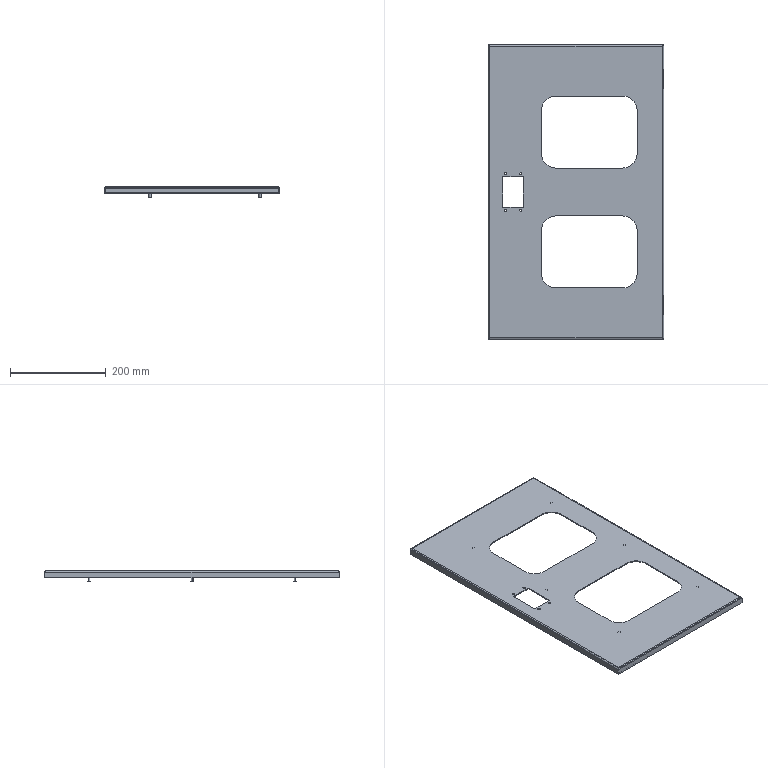Part | SolidWorks | features ICE 5, Fillet 2, Cut 1, Extrusion 1, HoleWzd 1, MirrorPattern 1, Shell 1 | 1 solid | 78 faces | box 365.5 x 614 x 22 mm | volume 439125 mm3 | plane 46 | cylinder 32 | commonest cylinder face diameters 6 x16 4.5 x8 60 x8